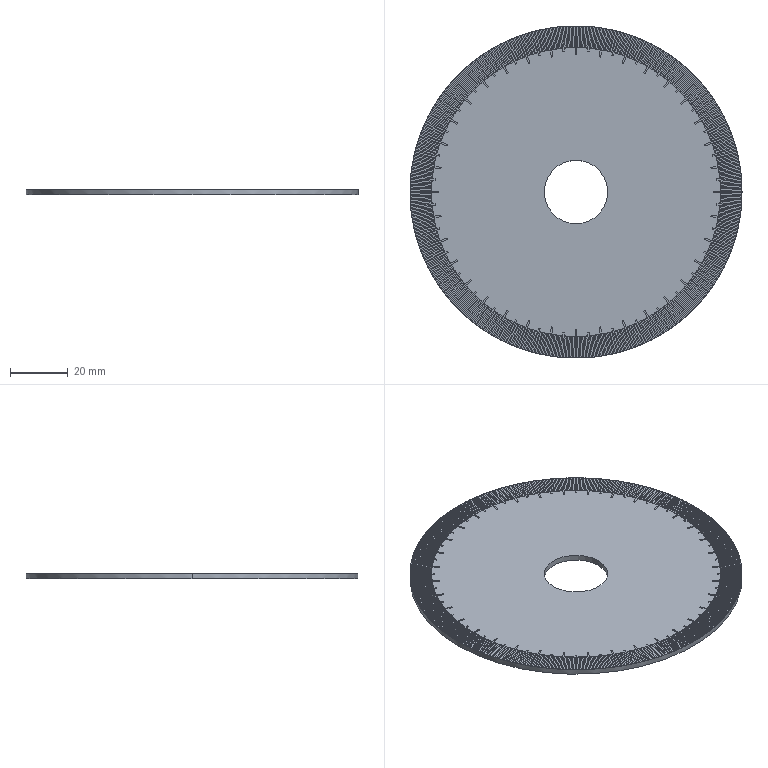Part | SolidWorks | features ICE 2, CirPattern 1, Extrusion 1 | 1 solid | 1483 faces | box 115 x 115 x 2 mm | volume 19943 mm3 | plane 1118 | cylinder 365 | commonest cylinder face diameters 100 x288 95 x37 98 x36 22 x2 115 x2